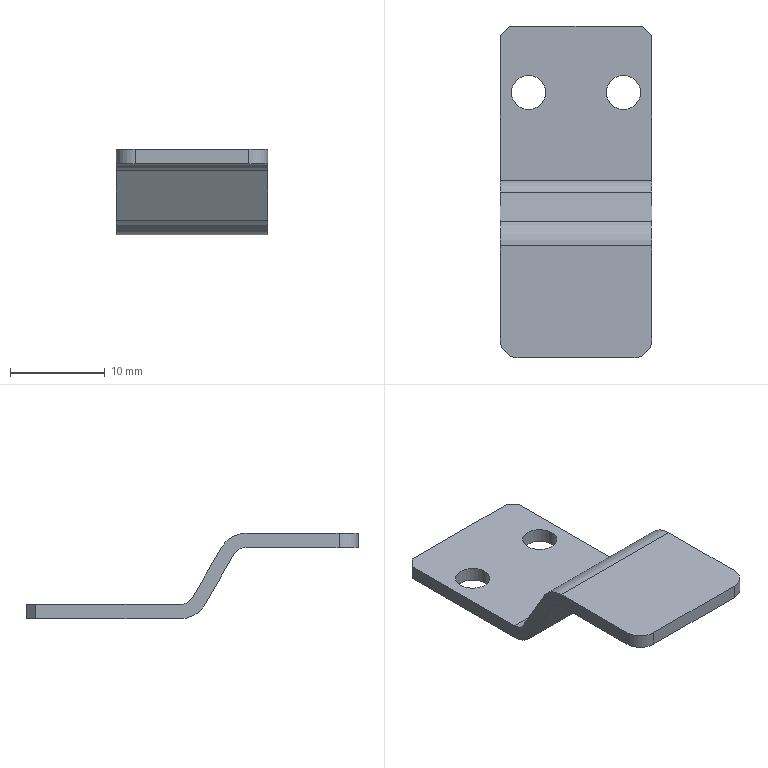Part | STEP file | 866-BDO024-93-10A | 1 solid | 22 faces | box 16 x 35 x 9 mm | volume 897.701 mm3 | plane 12 | cylinder 10 | commonest cylinder face diameters 3.6 x4 3 x2 4 x2 6 x2
STEP:
#1=CARTESIAN_POINT('',(-6.8,-7.,0.));
#2=VERTEX_POINT('',#1);
#3=CARTESIAN_POINT('',(-3.2,-7.,0.));
#4=VERTEX_POINT('',#3);
#5=CARTESIAN_POINT('',(-5.,-7.,0.));
#6=DIRECTION('',(0.,0.,1.));
#7=DIRECTION('',(1.,0.,0.));
#8=AXIS2_PLACEMENT_3D('',#5,#6,#7);
#9=CIRCLE('',#8,1.8);
#10=EDGE_CURVE('',#2,#4,#9,.T.);
#11=ORIENTED_EDGE('',*,*,#10,.F.);
#12=CARTESIAN_POINT('',(-6.8,-7.,1.5));
#13=VERTEX_POINT('',#12);
#14=CARTESIAN_POINT('',(-6.8,-7.,-0.001));
#15=DIRECTION('',(0.,0.,1.));
#16=VECTOR('',#15,1000.);
#17=LINE('',#14,#16);
#18=EDGE_CURVE('',#2,#13,#17,.T.);
#19=ORIENTED_EDGE('',*,*,#18,.T.);
#20=CARTESIAN_POINT('',(-3.2,-7.,1.5));
#21=VERTEX_POINT('',#20);
#22=CARTESIAN_POINT('',(-5.,-7.,1.5));
#23=DIRECTION('',(0.,0.,-1.));
#24=DIRECTION('',(1.,0.,0.));
#25=AXIS2_PLACEMENT_3D('',#22,#23,#24);
#26=CIRCLE('',#25,1.8);
#27=EDGE_CURVE('',#21,#13,#26,.T.);
#28=ORIENTED_EDGE('',*,*,#27,.F.);
#29=CARTESIAN_POINT('',(-3.2,-7.,-0.001));
#30=DIRECTION('',(0.,0.,1.));
#31=VECTOR('',#30,1000.);
#32=LINE('',#29,#31);
#33=EDGE_CURVE('',#4,#21,#32,.T.);
#34=ORIENTED_EDGE('',*,*,#33,.F.);
#35=EDGE_LOOP('',(#11,#19,#28,#34));
#36=FACE_OUTER_BOUND('',#35,.T.);
#37=CARTESIAN_POINT('',(-5.,-7.,-0.001));
#38=DIRECTION('',(0.,0.,1.));
#39=DIRECTION('',(1.,0.,0.));
#40=AXIS2_PLACEMENT_3D('',#37,#38,#39);
#41=CYLINDRICAL_SURFACE('',#40,1.8);
#42=ADVANCED_FACE('',(#36),#41,.F.);
#43=CARTESIAN_POINT('',(3.2,-7.,0.));
#44=VERTEX_POINT('',#43);
#45=CARTESIAN_POINT('',(6.8,-7.,0.));
#46=VERTEX_POINT('',#45);
#47=CARTESIAN_POINT('',(5.,-7.,0.));
#48=DIRECTION('',(0.,0.,1.));
#49=DIRECTION('',(1.,0.,0.));
#50=AXIS2_PLACEMENT_3D('',#47,#48,#49);
#51=CIRCLE('',#50,1.8);
#52=EDGE_CURVE('',#44,#46,#51,.T.);
#53=ORIENTED_EDGE('',*,*,#52,.F.);
#54=CARTESIAN_POINT('',(3.2,-7.,1.5));
#55=VERTEX_POINT('',#54);
#56=CARTESIAN_POINT('',(3.2,-7.,-0.001));
#57=DIRECTION('',(0.,0.,1.));
#58=VECTOR('',#57,1000.);
#59=LINE('',#56,#58);
#60=EDGE_CURVE('',#44,#55,#59,.T.);
#61=ORIENTED_EDGE('',*,*,#60,.T.);
#62=CARTESIAN_POINT('',(6.8,-7.,1.5));
#63=VERTEX_POINT('',#62);
#64=CARTESIAN_POINT('',(5.,-7.,1.5));
#65=DIRECTION('',(0.,0.,-1.));
#66=DIRECTION('',(1.,0.,0.));
#67=AXIS2_PLACEMENT_3D('',#64,#65,#66);
#68=CIRCLE('',#67,1.8);
#69=EDGE_CURVE('',#63,#55,#68,.T.);
#70=ORIENTED_EDGE('',*,*,#69,.F.);
#71=CARTESIAN_POINT('',(6.8,-7.,-0.001));
#72=DIRECTION('',(0.,0.,1.));
#73=VECTOR('',#72,1000.);
#74=LINE('',#71,#73);
#75=EDGE_CURVE('',#46,#63,#74,.T.);
#76=ORIENTED_EDGE('',*,*,#75,.F.);
#77=EDGE_LOOP('',(#53,#61,#70,#76));
#78=FACE_OUTER_BOUND('',#77,.T.);
#79=CARTESIAN_POINT('',(5.,-7.,-0.001));
#80=DIRECTION('',(0.,0.,1.));
#81=DIRECTION('',(1.,0.,0.));
#82=AXIS2_PLACEMENT_3D('',#79,#80,#81);
#83=CYLINDRICAL_SURFACE('',#82,1.8);
#84=ADVANCED_FACE('',(#78),#83,.F.);
#85=CARTESIAN_POINT('',(8.,-1.,0.));
#86=VERTEX_POINT('',#85);
#87=CARTESIAN_POINT('',(8.,-16.268,0.));
#88=VERTEX_POINT('',#87);
#89=CARTESIAN_POINT('',(8.,0.,0.));
#90=DIRECTION('',(0.,-1.,0.));
#91=VECTOR('',#90,1000.);
#92=LINE('',#89,#91);
#93=EDGE_CURVE('',#86,#88,#92,.T.);
#94=ORIENTED_EDGE('',*,*,#93,.T.);
#95=CARTESIAN_POINT('',(-8.,-16.268,0.));
#96=VERTEX_POINT('',#95);
#97=CARTESIAN_POINT('',(8.,-16.268,0.));
#98=DIRECTION('',(-1.,0.,0.));
#99=VECTOR('',#98,1000.);
#100=LINE('',#97,#99);
#101=EDGE_CURVE('',#88,#96,#100,.T.);
#102=ORIENTED_EDGE('',*,*,#101,.T.);
#103=CARTESIAN_POINT('',(-8.,-1.,0.));
#104=VERTEX_POINT('',#103);
#105=CARTESIAN_POINT('',(-8.,0.,0.));
#106=DIRECTION('',(0.,1.,0.));
#107=VECTOR('',#106,1000.);
#108=LINE('',#105,#107);
#109=EDGE_CURVE('',#96,#104,#108,.T.);
#110=ORIENTED_EDGE('',*,*,#109,.T.);
#111=CARTESIAN_POINT('',(-7.,0.,0.));
#112=VERTEX_POINT('',#111);
#113=CARTESIAN_POINT('',(-8.,-1.,0.));
#114=DIRECTION('',(0.7071,0.7071,0.));
#115=VECTOR('',#114,1000.);
#116=LINE('',#113,#115);
#117=EDGE_CURVE('',#104,#112,#116,.T.);
#118=ORIENTED_EDGE('',*,*,#117,.T.);
#119=CARTESIAN_POINT('',(7.,0.,0.));
#120=VERTEX_POINT('',#119);
#121=CARTESIAN_POINT('',(8.,0.,0.));
#122=DIRECTION('',(1.,0.,0.));
#123=VECTOR('',#122,1000.);
#124=LINE('',#121,#123);
#125=EDGE_CURVE('',#112,#120,#124,.T.);
#126=ORIENTED_EDGE('',*,*,#125,.T.);
#127=CARTESIAN_POINT('',(7.,0.,0.));
#128=DIRECTION('',(0.7071,-0.7071,0.));
#129=VECTOR('',#128,1000.);
#130=LINE('',#127,#129);
#131=EDGE_CURVE('',#120,#86,#130,.T.);
#132=ORIENTED_EDGE('',*,*,#131,.T.);
#133=EDGE_LOOP('',(#94,#102,#110,#118,#126,#132));
#134=FACE_OUTER_BOUND('',#133,.T.);
#135=CARTESIAN_POINT('',(-5.,-7.,0.));
#136=DIRECTION('',(0.,0.,1.));
#137=DIRECTION('',(1.,0.,0.));
#138=AXIS2_PLACEMENT_3D('',#135,#136,#137);
#139=CIRCLE('',#138,1.8);
#140=EDGE_CURVE('',#4,#2,#139,.T.);
#141=ORIENTED_EDGE('',*,*,#140,.T.);
#142=ORIENTED_EDGE('',*,*,#10,.T.);
#143=EDGE_LOOP('',(#141,#142));
#144=FACE_BOUND('',#143,.T.);
#145=CARTESIAN_POINT('',(5.,-7.,0.));
#146=DIRECTION('',(0.,0.,1.));
#147=DIRECTION('',(1.,0.,0.));
#148=AXIS2_PLACEMENT_3D('',#145,#146,#147);
#149=CIRCLE('',#148,1.8);
#150=EDGE_CURVE('',#46,#44,#149,.T.);
#151=ORIENTED_EDGE('',*,*,#150,.T.);
#152=ORIENTED_EDGE('',*,*,#52,.T.);
#153=EDGE_LOOP('',(#151,#152));
#154=FACE_BOUND('',#153,.T.);
#155=CARTESIAN_POINT('',(8.,0.,0.));
#156=DIRECTION('',(0.,0.,-1.));
#157=DIRECTION('',(0.,1.,0.));
#158=AXIS2_PLACEMENT_3D('',#155,#156,#157);
#159=PLANE('',#158);
#160=ADVANCED_FACE('',(#134,#144,#154),#159,.T.);
#161=CARTESIAN_POINT('',(8.,-18.866,1.5));
#162=VERTEX_POINT('',#161);
#163=CARTESIAN_POINT('',(8.,-16.268,3.));
#164=DIRECTION('',(-1.,0.,0.));
#165=DIRECTION('',(0.,0.,1.));
#166=AXIS2_PLACEMENT_3D('',#163,#164,#165);
#167=CIRCLE('',#166,3.);
#168=EDGE_CURVE('',#88,#162,#167,.T.);
#169=ORIENTED_EDGE('',*,*,#168,.T.);
#170=CARTESIAN_POINT('',(-8.,-18.866,1.5));
#171=VERTEX_POINT('',#170);
#172=CARTESIAN_POINT('',(8.,-18.866,1.5));
#173=DIRECTION('',(-1.,0.,0.));
#174=VECTOR('',#173,1000.);
#175=LINE('',#172,#174);
#176=EDGE_CURVE('',#162,#171,#175,.T.);
#177=ORIENTED_EDGE('',*,*,#176,.T.);
#178=CARTESIAN_POINT('',(-8.,-16.268,3.));
#179=DIRECTION('',(1.,0.,0.));
#180=DIRECTION('',(0.,0.,1.));
#181=AXIS2_PLACEMENT_3D('',#178,#179,#180);
#182=CIRCLE('',#181,3.);
#183=EDGE_CURVE('',#171,#96,#182,.T.);
#184=ORIENTED_EDGE('',*,*,#183,.T.);
#185=ORIENTED_EDGE('',*,*,#101,.F.);
#186=EDGE_LOOP('',(#169,#177,#184,#185));
#187=FACE_OUTER_BOUND('',#186,.T.);
#188=CARTESIAN_POINT('',(8.,-16.268,3.));
#189=DIRECTION('',(-1.,0.,0.));
#190=DIRECTION('',(0.,0.,1.));
#191=AXIS2_PLACEMENT_3D('',#188,#189,#190);
#192=CYLINDRICAL_SURFACE('',#191,3.);
#193=ADVANCED_FACE('',(#187),#192,.T.);
#194=CARTESIAN_POINT('',(8.,-1.,1.5));
#195=VERTEX_POINT('',#194);
#196=CARTESIAN_POINT('',(8.,-1.,6.));
#197=DIRECTION('',(0.,0.,-1.));
#198=VECTOR('',#197,1000.);
#199=LINE('',#196,#198);
#200=EDGE_CURVE('',#195,#86,#199,.T.);
#201=ORIENTED_EDGE('',*,*,#200,.F.);
#202=CARTESIAN_POINT('',(8.,-16.268,1.5));
#203=VERTEX_POINT('',#202);
#204=CARTESIAN_POINT('',(8.,-23.196,1.5));
#205=DIRECTION('',(0.,1.,0.));
#206=VECTOR('',#205,1000.);
#207=LINE('',#204,#206);
#208=EDGE_CURVE('',#203,#195,#207,.T.);
#209=ORIENTED_EDGE('',*,*,#208,.F.);
#210=CARTESIAN_POINT('',(8.,-17.567,2.25));
#211=VERTEX_POINT('',#210);
#212=CARTESIAN_POINT('',(8.,-16.268,3.));
#213=DIRECTION('',(-1.,0.,0.));
#214=DIRECTION('',(0.,0.,1.));
#215=AXIS2_PLACEMENT_3D('',#212,#213,#214);
#216=CIRCLE('',#215,1.5);
#217=EDGE_CURVE('',#203,#211,#216,.T.);
#218=ORIENTED_EDGE('',*,*,#217,.T.);
#219=CARTESIAN_POINT('',(8.,-20.598,7.5));
#220=VERTEX_POINT('',#219);
#221=CARTESIAN_POINT('',(8.,-17.567,2.25));
#222=DIRECTION('',(0.,-0.5,0.866));
#223=VECTOR('',#222,1000.);
#224=LINE('',#221,#223);
#225=EDGE_CURVE('',#211,#220,#224,.T.);
#226=ORIENTED_EDGE('',*,*,#225,.T.);
#227=CARTESIAN_POINT('',(8.,-23.196,9.));
#228=VERTEX_POINT('',#227);
#229=CARTESIAN_POINT('',(8.,-23.196,6.));
#230=DIRECTION('',(-1.,0.,0.));
#231=DIRECTION('',(0.,0.,1.));
#232=AXIS2_PLACEMENT_3D('',#229,#230,#231);
#233=CIRCLE('',#232,3.);
#234=EDGE_CURVE('',#228,#220,#233,.T.);
#235=ORIENTED_EDGE('',*,*,#234,.F.);
#236=CARTESIAN_POINT('',(8.,-33.,9.));
#237=VERTEX_POINT('',#236);
#238=CARTESIAN_POINT('',(8.,-20.598,9.));
#239=DIRECTION('',(0.,-1.,0.));
#240=VECTOR('',#239,1000.);
#241=LINE('',#238,#240);
#242=EDGE_CURVE('',#228,#237,#241,.T.);
#243=ORIENTED_EDGE('',*,*,#242,.T.);
#244=CARTESIAN_POINT('',(8.,-33.,7.5));
#245=VERTEX_POINT('',#244);
#246=CARTESIAN_POINT('',(8.,-33.,7.5));
#247=DIRECTION('',(0.,0.,1.));
#248=VECTOR('',#247,1000.);
#249=LINE('',#246,#248);
#250=EDGE_CURVE('',#245,#237,#249,.T.);
#251=ORIENTED_EDGE('',*,*,#250,.F.);
#252=CARTESIAN_POINT('',(8.,-23.196,7.5));
#253=VERTEX_POINT('',#252);
#254=CARTESIAN_POINT('',(8.,-22.33,7.5));
#255=DIRECTION('',(0.,-1.,0.));
#256=VECTOR('',#255,1000.);
#257=LINE('',#254,#256);
#258=EDGE_CURVE('',#253,#245,#257,.T.);
#259=ORIENTED_EDGE('',*,*,#258,.F.);
#260=CARTESIAN_POINT('',(8.,-21.897,6.75));
#261=VERTEX_POINT('',#260);
#262=CARTESIAN_POINT('',(8.,-23.196,6.));
#263=DIRECTION('',(-1.,0.,0.));
#264=DIRECTION('',(0.,0.,1.));
#265=AXIS2_PLACEMENT_3D('',#262,#263,#264);
#266=CIRCLE('',#265,1.5);
#267=EDGE_CURVE('',#253,#261,#266,.T.);
#268=ORIENTED_EDGE('',*,*,#267,.T.);
#269=CARTESIAN_POINT('',(8.,-18.,0.));
#270=DIRECTION('',(0.,-0.5,0.866));
#271=VECTOR('',#270,1000.);
#272=LINE('',#269,#271);
#273=EDGE_CURVE('',#162,#261,#272,.T.);
#274=ORIENTED_EDGE('',*,*,#273,.F.);
#275=ORIENTED_EDGE('',*,*,#168,.F.);
#276=ORIENTED_EDGE('',*,*,#93,.F.);
#277=EDGE_LOOP('',(#201,#209,#218,#226,#235,#243,#251,#259,#268,#274,#275,#276));
#278=FACE_OUTER_BOUND('',#277,.T.);
#279=CARTESIAN_POINT('',(8.,-23.196,6.));
#280=DIRECTION('',(-1.,0.,0.));
#281=DIRECTION('',(0.,0.,1.));
#282=AXIS2_PLACEMENT_3D('',#279,#280,#281);
#283=PLANE('',#282);
#284=ADVANCED_FACE('',(#278),#283,.F.);
#285=ORIENTED_EDGE('',*,*,#131,.F.);
#286=CARTESIAN_POINT('',(7.,0.,1.5));
#287=VERTEX_POINT('',#286);
#288=CARTESIAN_POINT('',(7.,0.,1.5));
#289=DIRECTION('',(0.,0.,1.));
#290=VECTOR('',#289,1000.);
#291=LINE('',#288,#290);
#292=EDGE_CURVE('',#120,#287,#291,.T.);
#293=ORIENTED_EDGE('',*,*,#292,.T.);
#294=CARTESIAN_POINT('',(7.,0.,1.5));
#295=DIRECTION('',(0.7071,-0.7071,0.));
#296=VECTOR('',#295,1000.);
#297=LINE('',#294,#296);
#298=EDGE_CURVE('',#287,#195,#297,.T.);
#299=ORIENTED_EDGE('',*,*,#298,.T.);
#300=ORIENTED_EDGE('',*,*,#200,.T.);
#301=EDGE_LOOP('',(#285,#293,#299,#300));
#302=FACE_OUTER_BOUND('',#301,.T.);
#303=CARTESIAN_POINT('',(7.,0.,1.5));
#304=DIRECTION('',(0.7071,0.7071,0.));
#305=DIRECTION('',(-0.7071,0.7071,0.));
#306=AXIS2_PLACEMENT_3D('',#303,#304,#305);
#307=PLANE('',#306);
#308=ADVANCED_FACE('',(#302),#307,.T.);
#309=CARTESIAN_POINT('',(-7.,0.,1.5));
#310=VERTEX_POINT('',#309);
#311=CARTESIAN_POINT('',(8.,0.,1.5));
#312=DIRECTION('',(1.,0.,0.));
#313=VECTOR('',#312,1000.);
#314=LINE('',#311,#313);
#315=EDGE_CURVE('',#310,#287,#314,.T.);
#316=ORIENTED_EDGE('',*,*,#315,.T.);
#317=ORIENTED_EDGE('',*,*,#292,.F.);
#318=ORIENTED_EDGE('',*,*,#125,.F.);
#319=CARTESIAN_POINT('',(-7.,0.,1.5));
#320=DIRECTION('',(0.,0.,1.));
#321=VECTOR('',#320,1000.);
#322=LINE('',#319,#321);
#323=EDGE_CURVE('',#112,#310,#322,.T.);
#324=ORIENTED_EDGE('',*,*,#323,.T.);
#325=EDGE_LOOP('',(#316,#317,#318,#324));
#326=FACE_OUTER_BOUND('',#325,.T.);
#327=CARTESIAN_POINT('',(8.,0.,1.5));
#328=DIRECTION('',(0.,1.,0.));
#329=DIRECTION('',(0.,0.,1.));
#330=AXIS2_PLACEMENT_3D('',#327,#328,#329);
#331=PLANE('',#330);
#332=ADVANCED_FACE('',(#326),#331,.T.);
#333=ORIENTED_EDGE('',*,*,#323,.F.);
#334=ORIENTED_EDGE('',*,*,#117,.F.);
#335=CARTESIAN_POINT('',(-8.,-1.,1.5));
#336=VERTEX_POINT('',#335);
#337=CARTESIAN_POINT('',(-8.,-1.,2.25));
#338=DIRECTION('',(0.,0.,-1.));
#339=VECTOR('',#338,1000.);
#340=LINE('',#337,#339);
#341=EDGE_CURVE('',#336,#104,#340,.T.);
#342=ORIENTED_EDGE('',*,*,#341,.F.);
#343=CARTESIAN_POINT('',(-8.,-1.,1.5));
#344=DIRECTION('',(-0.7071,-0.7071,0.));
#345=VECTOR('',#344,1000.);
#346=LINE('',#343,#345);
#347=EDGE_CURVE('',#310,#336,#346,.T.);
#348=ORIENTED_EDGE('',*,*,#347,.F.);
#349=EDGE_LOOP('',(#333,#334,#342,#348));
#350=FACE_OUTER_BOUND('',#349,.T.);
#351=CARTESIAN_POINT('',(-8.,-1.,2.25));
#352=DIRECTION('',(0.7071,-0.7071,0.));
#353=DIRECTION('',(0.7071,0.7071,0.));
#354=AXIS2_PLACEMENT_3D('',#351,#352,#353);
#355=PLANE('',#354);
#356=ADVANCED_FACE('',(#350),#355,.F.);
#357=ORIENTED_EDGE('',*,*,#109,.F.);
#358=ORIENTED_EDGE('',*,*,#183,.F.);
#359=CARTESIAN_POINT('',(-8.,-21.897,6.75));
#360=VERTEX_POINT('',#359);
#361=CARTESIAN_POINT('',(-8.,-18.,0.));
#362=DIRECTION('',(0.,0.5,-0.866));
#363=VECTOR('',#362,1000.);
#364=LINE('',#361,#363);
#365=EDGE_CURVE('',#360,#171,#364,.T.);
#366=ORIENTED_EDGE('',*,*,#365,.F.);
#367=CARTESIAN_POINT('',(-8.,-23.196,7.5));
#368=VERTEX_POINT('',#367);
#369=CARTESIAN_POINT('',(-8.,-23.196,6.));
#370=DIRECTION('',(1.,0.,0.));
#371=DIRECTION('',(0.,0.,1.));
#372=AXIS2_PLACEMENT_3D('',#369,#370,#371);
#373=CIRCLE('',#372,1.5);
#374=EDGE_CURVE('',#360,#368,#373,.T.);
#375=ORIENTED_EDGE('',*,*,#374,.T.);
#376=CARTESIAN_POINT('',(-8.,-33.,7.5));
#377=VERTEX_POINT('',#376);
#378=CARTESIAN_POINT('',(-8.,-22.33,7.5));
#379=DIRECTION('',(0.,1.,0.));
#380=VECTOR('',#379,1000.);
#381=LINE('',#378,#380);
#382=EDGE_CURVE('',#377,#368,#381,.T.);
#383=ORIENTED_EDGE('',*,*,#382,.F.);
#384=CARTESIAN_POINT('',(-8.,-33.,9.));
#385=VERTEX_POINT('',#384);
#386=CARTESIAN_POINT('',(-8.,-33.,6.));
#387=DIRECTION('',(0.,0.,1.));
#388=VECTOR('',#387,1000.);
#389=LINE('',#386,#388);
#390=EDGE_CURVE('',#377,#385,#389,.T.);
#391=ORIENTED_EDGE('',*,*,#390,.T.);
#392=CARTESIAN_POINT('',(-8.,-23.196,9.));
#393=VERTEX_POINT('',#392);
#394=CARTESIAN_POINT('',(-8.,-23.196,9.));
#395=DIRECTION('',(0.,1.,0.));
#396=VECTOR('',#395,1000.);
#397=LINE('',#394,#396);
#398=EDGE_CURVE('',#385,#393,#397,.T.);
#399=ORIENTED_EDGE('',*,*,#398,.T.);
#400=CARTESIAN_POINT('',(-8.,-20.598,7.5));
#401=VERTEX_POINT('',#400);
#402=CARTESIAN_POINT('',(-8.,-23.196,6.));
#403=DIRECTION('',(1.,0.,0.));
#404=DIRECTION('',(0.,0.,1.));
#405=AXIS2_PLACEMENT_3D('',#402,#403,#404);
#406=CIRCLE('',#405,3.);
#407=EDGE_CURVE('',#401,#393,#406,.T.);
#408=ORIENTED_EDGE('',*,*,#407,.F.);
#409=CARTESIAN_POINT('',(-8.,-17.567,2.25));
#410=VERTEX_POINT('',#409);
#411=CARTESIAN_POINT('',(-8.,-20.598,7.5));
#412=DIRECTION('',(0.,0.5,-0.866));
#413=VECTOR('',#412,1000.);
#414=LINE('',#411,#413);
#415=EDGE_CURVE('',#401,#410,#414,.T.);
#416=ORIENTED_EDGE('',*,*,#415,.T.);
#417=CARTESIAN_POINT('',(-8.,-16.268,1.5));
#418=VERTEX_POINT('',#417);
#419=CARTESIAN_POINT('',(-8.,-16.268,3.));
#420=DIRECTION('',(1.,0.,0.));
#421=DIRECTION('',(0.,0.,1.));
#422=AXIS2_PLACEMENT_3D('',#419,#420,#421);
#423=CIRCLE('',#422,1.5);
#424=EDGE_CURVE('',#410,#418,#423,.T.);
#425=ORIENTED_EDGE('',*,*,#424,.T.);
#426=CARTESIAN_POINT('',(-8.,-17.567,1.5));
#427=DIRECTION('',(0.,1.,0.));
#428=VECTOR('',#427,1000.);
#429=LINE('',#426,#428);
#430=EDGE_CURVE('',#418,#336,#429,.T.);
#431=ORIENTED_EDGE('',*,*,#430,.T.);
#432=ORIENTED_EDGE('',*,*,#341,.T.);
#433=EDGE_LOOP('',(#357,#358,#366,#375,#383,#391,#399,#408,#416,#425,#431,#432));
#434=FACE_OUTER_BOUND('',#433,.T.);
#435=CARTESIAN_POINT('',(-8.,-17.567,2.25));
#436=DIRECTION('',(-1.,0.,0.));
#437=DIRECTION('',(0.,0.,1.));
#438=AXIS2_PLACEMENT_3D('',#435,#436,#437);
#439=PLANE('',#438);
#440=ADVANCED_FACE('',(#434),#439,.T.);
#441=ORIENTED_EDGE('',*,*,#18,.F.);
#442=ORIENTED_EDGE('',*,*,#140,.F.);
#443=ORIENTED_EDGE('',*,*,#33,.T.);
#444=CARTESIAN_POINT('',(-5.,-7.,1.5));
#445=DIRECTION('',(0.,0.,-1.));
#446=DIRECTION('',(1.,0.,0.));
#447=AXIS2_PLACEMENT_3D('',#444,#445,#446);
#448=CIRCLE('',#447,1.8);
#449=EDGE_CURVE('',#13,#21,#448,.T.);
#450=ORIENTED_EDGE('',*,*,#449,.F.);
#451=EDGE_LOOP('',(#441,#442,#443,#450));
#452=FACE_OUTER_BOUND('',#451,.T.);
#453=CARTESIAN_POINT('',(-5.,-7.,-0.001));
#454=DIRECTION('',(0.,0.,1.));
#455=DIRECTION('',(1.,0.,0.));
#456=AXIS2_PLACEMENT_3D('',#453,#454,#455);
#457=CYLINDRICAL_SURFACE('',#456,1.8);
#458=ADVANCED_FACE('',(#452),#457,.F.);
#459=ORIENTED_EDGE('',*,*,#60,.F.);
#460=ORIENTED_EDGE('',*,*,#150,.F.);
#461=ORIENTED_EDGE('',*,*,#75,.T.);
#462=CARTESIAN_POINT('',(5.,-7.,1.5));
#463=DIRECTION('',(0.,0.,-1.));
#464=DIRECTION('',(1.,0.,0.));
#465=AXIS2_PLACEMENT_3D('',#462,#463,#464);
#466=CIRCLE('',#465,1.8);
#467=EDGE_CURVE('',#55,#63,#466,.T.);
#468=ORIENTED_EDGE('',*,*,#467,.F.);
#469=EDGE_LOOP('',(#459,#460,#461,#468));
#470=FACE_OUTER_BOUND('',#469,.T.);
#471=CARTESIAN_POINT('',(5.,-7.,-0.001));
#472=DIRECTION('',(0.,0.,1.));
#473=DIRECTION('',(1.,0.,0.));
#474=AXIS2_PLACEMENT_3D('',#471,#472,#473);
#475=CYLINDRICAL_SURFACE('',#474,1.8);
#476=ADVANCED_FACE('',(#470),#475,.F.);
#477=ORIENTED_EDGE('',*,*,#273,.T.);
#478=CARTESIAN_POINT('',(8.,-21.897,6.75));
#479=DIRECTION('',(-1.,0.,0.));
#480=VECTOR('',#479,1000.);
#481=LINE('',#478,#480);
#482=EDGE_CURVE('',#261,#360,#481,.T.);
#483=ORIENTED_EDGE('',*,*,#482,.T.);
#484=ORIENTED_EDGE('',*,*,#365,.T.);
#485=ORIENTED_EDGE('',*,*,#176,.F.);
#486=EDGE_LOOP('',(#477,#483,#484,#485));
#487=FACE_OUTER_BOUND('',#486,.T.);
#488=CARTESIAN_POINT('',(8.,-18.,0.));
#489=DIRECTION('',(0.,-0.866,-0.5));
#490=DIRECTION('',(0.,0.5,-0.866));
#491=AXIS2_PLACEMENT_3D('',#488,#489,#490);
#492=PLANE('',#491);
#493=ADVANCED_FACE('',(#487),#492,.T.);
#494=ORIENTED_EDGE('',*,*,#347,.T.);
#495=ORIENTED_EDGE('',*,*,#430,.F.);
#496=CARTESIAN_POINT('',(8.,-16.268,1.5));
#497=DIRECTION('',(-1.,0.,0.));
#498=VECTOR('',#497,1000.);
#499=LINE('',#496,#498);
#500=EDGE_CURVE('',#203,#418,#499,.T.);
#501=ORIENTED_EDGE('',*,*,#500,.F.);
#502=ORIENTED_EDGE('',*,*,#208,.T.);
#503=ORIENTED_EDGE('',*,*,#298,.F.);
#504=ORIENTED_EDGE('',*,*,#315,.F.);
#505=EDGE_LOOP('',(#494,#495,#501,#502,#503,#504));
#506=FACE_OUTER_BOUND('',#505,.T.);
#507=ORIENTED_EDGE('',*,*,#27,.T.);
#508=ORIENTED_EDGE('',*,*,#449,.T.);
#509=EDGE_LOOP('',(#507,#508));
#510=FACE_BOUND('',#509,.T.);
#511=ORIENTED_EDGE('',*,*,#69,.T.);
#512=ORIENTED_EDGE('',*,*,#467,.T.);
#513=EDGE_LOOP('',(#511,#512));
#514=FACE_BOUND('',#513,.T.);
#515=CARTESIAN_POINT('',(8.,0.,1.5));
#516=DIRECTION('',(0.,0.,-1.));
#517=DIRECTION('',(0.,1.,0.));
#518=AXIS2_PLACEMENT_3D('',#515,#516,#517);
#519=PLANE('',#518);
#520=ADVANCED_FACE('',(#506,#510,#514),#519,.F.);
#521=ORIENTED_EDGE('',*,*,#482,.F.);
#522=ORIENTED_EDGE('',*,*,#267,.F.);
#523=CARTESIAN_POINT('',(8.,-23.196,7.5));
#524=DIRECTION('',(1.,0.,0.));
#525=VECTOR('',#524,1000.);
#526=LINE('',#523,#525);
#527=EDGE_CURVE('',#368,#253,#526,.T.);
#528=ORIENTED_EDGE('',*,*,#527,.F.);
#529=ORIENTED_EDGE('',*,*,#374,.F.);
#530=EDGE_LOOP('',(#521,#522,#528,#529));
#531=FACE_OUTER_BOUND('',#530,.T.);
#532=CARTESIAN_POINT('',(8.,-23.196,6.));
#533=DIRECTION('',(-1.,0.,0.));
#534=DIRECTION('',(0.,0.,1.));
#535=AXIS2_PLACEMENT_3D('',#532,#533,#534);
#536=CYLINDRICAL_SURFACE('',#535,1.5);
#537=ADVANCED_FACE('',(#531),#536,.F.);
#538=CARTESIAN_POINT('',(8.,-17.567,2.25));
#539=DIRECTION('',(-1.,0.,0.));
#540=VECTOR('',#539,1000.);
#541=LINE('',#538,#540);
#542=EDGE_CURVE('',#211,#410,#541,.T.);
#543=ORIENTED_EDGE('',*,*,#542,.F.);
#544=ORIENTED_EDGE('',*,*,#217,.F.);
#545=ORIENTED_EDGE('',*,*,#500,.T.);
#546=ORIENTED_EDGE('',*,*,#424,.F.);
#547=EDGE_LOOP('',(#543,#544,#545,#546));
#548=FACE_OUTER_BOUND('',#547,.T.);
#549=CARTESIAN_POINT('',(8.,-16.268,3.));
#550=DIRECTION('',(-1.,0.,0.));
#551=DIRECTION('',(0.,0.,1.));
#552=AXIS2_PLACEMENT_3D('',#549,#550,#551);
#553=CYLINDRICAL_SURFACE('',#552,1.5);
#554=ADVANCED_FACE('',(#548),#553,.F.);
#555=ORIENTED_EDGE('',*,*,#258,.T.);
#556=CARTESIAN_POINT('',(6.,-35.,7.5));
#557=VERTEX_POINT('',#556);
#558=CARTESIAN_POINT('',(6.,-33.,7.5));
#559=DIRECTION('',(0.,0.,-1.));
#560=DIRECTION('',(1.,0.,0.));
#561=AXIS2_PLACEMENT_3D('',#558,#559,#560);
#562=CIRCLE('',#561,2.);
#563=EDGE_CURVE('',#245,#557,#562,.T.);
#564=ORIENTED_EDGE('',*,*,#563,.T.);
#565=CARTESIAN_POINT('',(-6.,-35.,7.5));
#566=VERTEX_POINT('',#565);
#567=CARTESIAN_POINT('',(8.,-35.,7.5));
#568=DIRECTION('',(-1.,0.,0.));
#569=VECTOR('',#568,1000.);
#570=LINE('',#567,#569);
#571=EDGE_CURVE('',#557,#566,#570,.T.);
#572=ORIENTED_EDGE('',*,*,#571,.T.);
#573=CARTESIAN_POINT('',(-6.,-33.,7.5));
#574=DIRECTION('',(0.,0.,-1.));
#575=DIRECTION('',(1.,0.,0.));
#576=AXIS2_PLACEMENT_3D('',#573,#574,#575);
#577=CIRCLE('',#576,2.);
#578=EDGE_CURVE('',#566,#377,#577,.T.);
#579=ORIENTED_EDGE('',*,*,#578,.T.);
#580=ORIENTED_EDGE('',*,*,#382,.T.);
#581=ORIENTED_EDGE('',*,*,#527,.T.);
#582=EDGE_LOOP('',(#555,#564,#572,#579,#580,#581));
#583=FACE_OUTER_BOUND('',#582,.T.);
#584=CARTESIAN_POINT('',(8.,-22.33,7.5));
#585=DIRECTION('',(0.,0.,-1.));
#586=DIRECTION('',(0.,1.,0.));
#587=AXIS2_PLACEMENT_3D('',#584,#585,#586);
#588=PLANE('',#587);
#589=ADVANCED_FACE('',(#583),#588,.T.);
#590=CARTESIAN_POINT('',(8.,-20.598,7.5));
#591=DIRECTION('',(-1.,0.,0.));
#592=VECTOR('',#591,1000.);
#593=LINE('',#590,#592);
#594=EDGE_CURVE('',#220,#401,#593,.T.);
#595=ORIENTED_EDGE('',*,*,#594,.F.);
#596=ORIENTED_EDGE('',*,*,#225,.F.);
#597=ORIENTED_EDGE('',*,*,#542,.T.);
#598=ORIENTED_EDGE('',*,*,#415,.F.);
#599=EDGE_LOOP('',(#595,#596,#597,#598));
#600=FACE_OUTER_BOUND('',#599,.T.);
#601=CARTESIAN_POINT('',(8.,-16.701,0.75));
#602=DIRECTION('',(0.,-0.866,-0.5));
#603=DIRECTION('',(0.,0.5,-0.866));
#604=AXIS2_PLACEMENT_3D('',#601,#602,#603);
#605=PLANE('',#604);
#606=ADVANCED_FACE('',(#600),#605,.F.);
#607=CARTESIAN_POINT('',(6.,-35.,9.));
#608=VERTEX_POINT('',#607);
#609=CARTESIAN_POINT('',(6.,-33.,9.));
#610=DIRECTION('',(0.,0.,-1.));
#611=DIRECTION('',(1.,0.,0.));
#612=AXIS2_PLACEMENT_3D('',#609,#610,#611);
#613=CIRCLE('',#612,2.);
#614=EDGE_CURVE('',#237,#608,#613,.T.);
#615=ORIENTED_EDGE('',*,*,#614,.T.);
#616=CARTESIAN_POINT('',(6.,-35.,7.5));
#617=DIRECTION('',(0.,0.,-1.));
#618=VECTOR('',#617,1000.);
#619=LINE('',#616,#618);
#620=EDGE_CURVE('',#608,#557,#619,.T.);
#621=ORIENTED_EDGE('',*,*,#620,.T.);
#622=ORIENTED_EDGE('',*,*,#563,.F.);
#623=ORIENTED_EDGE('',*,*,#250,.T.);
#624=EDGE_LOOP('',(#615,#621,#622,#623));
#625=FACE_OUTER_BOUND('',#624,.T.);
#626=CARTESIAN_POINT('',(6.,-33.,7.5));
#627=DIRECTION('',(0.,0.,1.));
#628=DIRECTION('',(1.,0.,0.));
#629=AXIS2_PLACEMENT_3D('',#626,#627,#628);
#630=CYLINDRICAL_SURFACE('',#629,2.);
#631=ADVANCED_FACE('',(#625),#630,.T.);
#632=CARTESIAN_POINT('',(-6.,-35.,9.));
#633=VERTEX_POINT('',#632);
#634=CARTESIAN_POINT('',(-6.,-33.,9.));
#635=DIRECTION('',(0.,0.,-1.));
#636=DIRECTION('',(1.,0.,0.));
#637=AXIS2_PLACEMENT_3D('',#634,#635,#636);
#638=CIRCLE('',#637,2.);
#639=EDGE_CURVE('',#633,#385,#638,.T.);
#640=ORIENTED_EDGE('',*,*,#639,.T.);
#641=ORIENTED_EDGE('',*,*,#390,.F.);
#642=ORIENTED_EDGE('',*,*,#578,.F.);
#643=CARTESIAN_POINT('',(-6.,-35.,6.));
#644=DIRECTION('',(0.,0.,1.));
#645=VECTOR('',#644,1000.);
#646=LINE('',#643,#645);
#647=EDGE_CURVE('',#566,#633,#646,.T.);
#648=ORIENTED_EDGE('',*,*,#647,.T.);
#649=EDGE_LOOP('',(#640,#641,#642,#648));
#650=FACE_OUTER_BOUND('',#649,.T.);
#651=CARTESIAN_POINT('',(-6.,-33.,6.));
#652=DIRECTION('',(0.,0.,1.));
#653=DIRECTION('',(1.,0.,0.));
#654=AXIS2_PLACEMENT_3D('',#651,#652,#653);
#655=CYLINDRICAL_SURFACE('',#654,2.);
#656=ADVANCED_FACE('',(#650),#655,.T.);
#657=ORIENTED_EDGE('',*,*,#571,.F.);
#658=ORIENTED_EDGE('',*,*,#620,.F.);
#659=CARTESIAN_POINT('',(8.,-35.,9.));
#660=DIRECTION('',(-1.,0.,0.));
#661=VECTOR('',#660,1000.);
#662=LINE('',#659,#661);
#663=EDGE_CURVE('',#608,#633,#662,.T.);
#664=ORIENTED_EDGE('',*,*,#663,.T.);
#665=ORIENTED_EDGE('',*,*,#647,.F.);
#666=EDGE_LOOP('',(#657,#658,#664,#665));
#667=FACE_OUTER_BOUND('',#666,.T.);
#668=CARTESIAN_POINT('',(8.,-35.,7.5));
#669=DIRECTION('',(0.,-1.,0.));
#670=DIRECTION('',(0.,0.,-1.));
#671=AXIS2_PLACEMENT_3D('',#668,#669,#670);
#672=PLANE('',#671);
#673=ADVANCED_FACE('',(#667),#672,.T.);
#674=ORIENTED_EDGE('',*,*,#234,.T.);
#675=ORIENTED_EDGE('',*,*,#594,.T.);
#676=ORIENTED_EDGE('',*,*,#407,.T.);
#677=CARTESIAN_POINT('',(8.,-23.196,9.));
#678=DIRECTION('',(1.,0.,0.));
#679=VECTOR('',#678,1000.);
#680=LINE('',#677,#679);
#681=EDGE_CURVE('',#393,#228,#680,.T.);
#682=ORIENTED_EDGE('',*,*,#681,.T.);
#683=EDGE_LOOP('',(#674,#675,#676,#682));
#684=FACE_OUTER_BOUND('',#683,.T.);
#685=CARTESIAN_POINT('',(8.,-23.196,6.));
#686=DIRECTION('',(-1.,0.,0.));
#687=DIRECTION('',(0.,0.,1.));
#688=AXIS2_PLACEMENT_3D('',#685,#686,#687);
#689=CYLINDRICAL_SURFACE('',#688,3.);
#690=ADVANCED_FACE('',(#684),#689,.T.);
#691=ORIENTED_EDGE('',*,*,#639,.F.);
#692=ORIENTED_EDGE('',*,*,#663,.F.);
#693=ORIENTED_EDGE('',*,*,#614,.F.);
#694=ORIENTED_EDGE('',*,*,#242,.F.);
#695=ORIENTED_EDGE('',*,*,#681,.F.);
#696=ORIENTED_EDGE('',*,*,#398,.F.);
#697=EDGE_LOOP('',(#691,#692,#693,#694,#695,#696));
#698=FACE_OUTER_BOUND('',#697,.T.);
#699=CARTESIAN_POINT('',(8.,-22.33,9.));
#700=DIRECTION('',(0.,0.,-1.));
#701=DIRECTION('',(0.,1.,0.));
#702=AXIS2_PLACEMENT_3D('',#699,#700,#701);
#703=PLANE('',#702);
#704=ADVANCED_FACE('',(#698),#703,.F.);
#705=CLOSED_SHELL('',(#42,#84,#160,#193,#284,#308,#332,#356,#440,#458,#476,#493,#520,#537,#554,#589,#606,#631,#656,#673,#690,#704));
#706=MANIFOLD_SOLID_BREP('',#705);
#707=CARTESIAN_POINT('',(0.,0.,0.));
#708=DIRECTION('',(0.,0.,1.));
#709=DIRECTION('',(1.,0.,0.));
#710=AXIS2_PLACEMENT_3D('',#707,#708,#709);
#711=(LENGTH_UNIT()NAMED_UNIT(*)SI_UNIT(.MILLI.,.METRE.));
#712=UNCERTAINTY_MEASURE_WITH_UNIT(LENGTH_MEASURE(0.00001),#711,'','');
#713=(NAMED_UNIT(*)PLANE_ANGLE_UNIT()SI_UNIT($,.RADIAN.));
#714=(NAMED_UNIT(*)SI_UNIT($,.STERADIAN.)SOLID_ANGLE_UNIT());
#715=(GEOMETRIC_REPRESENTATION_CONTEXT(3)GLOBAL_UNCERTAINTY_ASSIGNED_CONTEXT((#712))GLOBAL_UNIT_ASSIGNED_CONTEXT((#711,#713,#714))REPRESENTATION_CONTEXT('',''));
#716=ADVANCED_BREP_SHAPE_REPRESENTATION('',(#706,#710),#715);